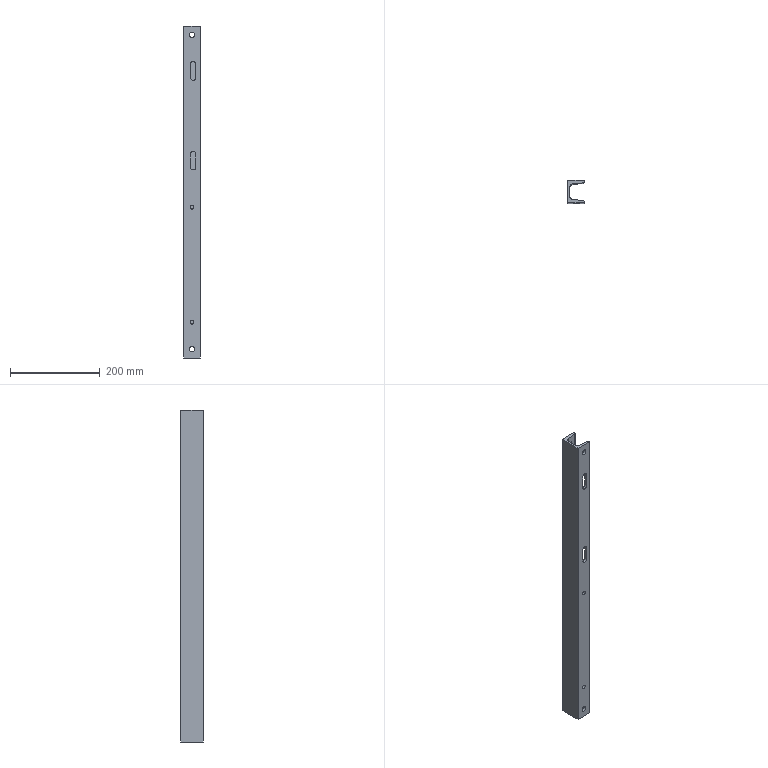Part | STEP file | HESS-408-70-15W-W-41-5# channel 3_default_machined_ | 1 solid | 34 faces | box 37 x 50 x 740 mm | volume 491245 mm3 | cylinder 20 | plane 14 | commonest cylinder face diameters 12 x12 8.5 x4 7 x2 14 x2